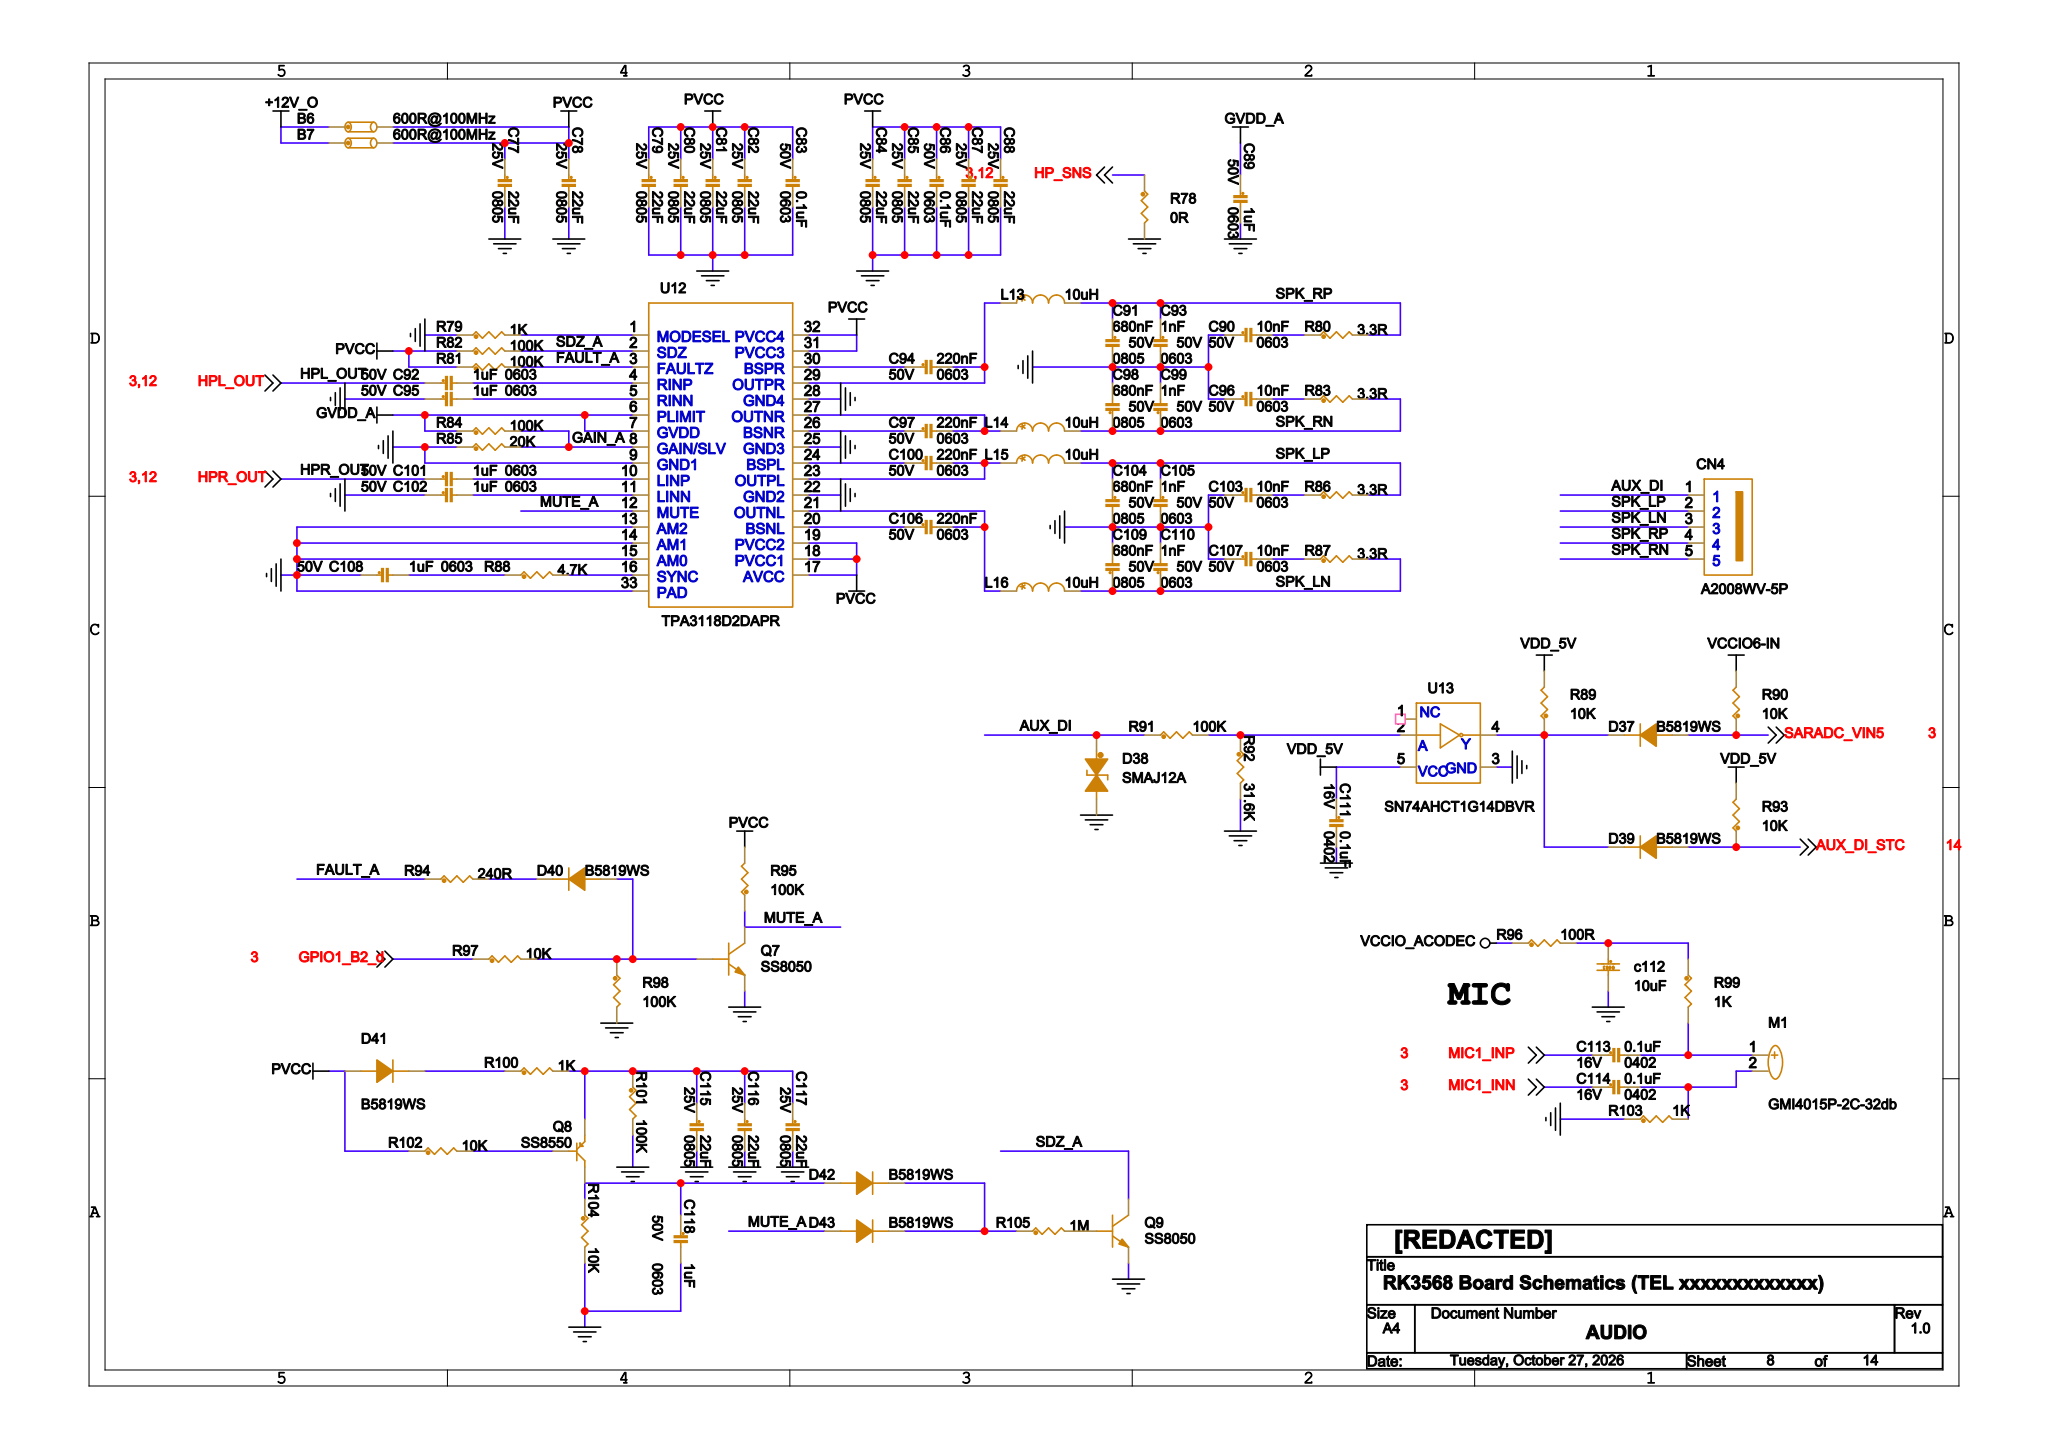Circuit board | Cadence Allegro | 669 parts | 581 nets | one sheet of the schematic
Parts on this sheet (reference | value | footprint):
B6 | 600R@100MHz | R0805
B7 | 600R@100MHz | R0805
C77 | 22uF | C0805
C78 | 22uF | C0805
C79 | 22uF | C0805
C80 | 22uF | C0805
C81 | 22uF | C0805
C82 | 22uF | C0805
C83 | 0.1uF | C0603
C84 | 22uF | C0805
C85 | 22uF | C0805
C86 | 0.1uF | C0603
C87 | 22uF | C0805
C88 | 22uF | C0805
C89 | 1uF | C0603
C90 | 10nF | C0603
C91 | 680nF | C0805
C92 | 1uF | C0603
C93 | 1nF | C0603
C94 | 220nF | C0603
C95 | 1uF | C0603
C96 | 10nF | C0603
C97 | 220nF | C0603
C98 | 680nF | C0805
C99 | 1nF | C0603
C100 | 220nF | C0603
C101 | 1uF | C0603
C102 | 1uF | C0603
C103 | 10nF | C0603
C104 | 680nF | C0805
C105 | 1nF | C0603
C106 | 220nF | C0603
C107 | 10nF | C0603
C108 | 1uF | C0603
C109 | 680nF | C0805
C110 | 1nF | C0603
C111 | 0.1uF | C0402
C113 | 0.1uF | C0402
C114 | 0.1uF | C0402
C115 | 22uF | C0805
C116 | 22uF | C0805
C117 | 22uF | C0805
C118 | 1uF | C0603
CN4 | A2008WV-5P | A2008WV_5P
D37 | B5819WS | SOD323
D38 | SMAJ12A | SMA
D39 | B5819WS | SOD323
D40 | B5819WS | SOD323
D41 | B5819WS | SOD323
D42 | B5819WS | SOD323
D43 | B5819WS | SOD323
L13 | 10uH | IND0630
L14 | 10uH | IND0630
L15 | 10uH | IND0630
L16 | 10uH | IND0630
M1 | GMI4015P-2C-32db | MIC4015P
Q7 | SS8050 | SOT-23
Q8 | SS8550 | SOT-23
Q9 | SS8050 | SOT-23
R78 | 0R | R0402
R79 | 1K | R0402
R80 | 3.3R | R0603
R81 | 100K | R0402
R82 | 100K | R0402
R83 | 3.3R | R0603
R84 | 100K | R0402
R85 | 20K | R0402
R86 | 3.3R | R0603
R87 | 3.3R | R0603
R88 | 4.7K | R0402
R89 | 10K | R0402
R90 | 10K | R0402
R91 | 100K | R0402
R92 | 31.6K | R0402
R93 | 10K | R0402
R94 | 240R | R0402
R95 | 100K | R0402
R96 | 100R | R0402
R97 | 10K | R0402
R98 | 100K | R0402
R99 | 1K | R0402
R100 | 1K | R0402
R101 | 100K | R0402
R102 | 10K | R0402
R103 | 1K | R0402
R104 | 10K | R0402
R105 | 1M | R0402
U12 | TPA3118D2DAPR | HTSSOP32
U13 | SN74AHCT1G14DBVR | SOT23-5
Nets of these parts (net: part-pin ...):
GND: C77-2 C78-2 C79-2 C80-2 C81-2 C82-2 C83-2 C84-2 C85-2 C86-2 C87-2 C88-2 C89-2 C90-1 C91-2 C93-2 C95-1 C96-1 C98-2 C99-2 C102-1 C103-1 C104-2 C105-2 C107-1 C108-1 C109-2 C110-2 C111-2 C115-2 C116-2 C117-2 C118-2 D38-1 Q7-2 Q9-2 R78-2 R79-1 R85-1 R92-2 R98-2 R101-2 R103-1 R104-2 U13-3 U12-9 U12-13 U12-14 U12-15 U12-22 U12-25 U12-28 U12-33
VDD_5V: C111-1 R89-2 R93-2 U13-5
+12V_O: B6-1 B7-1
SARADC_VIN5: D37-1 R90-1
N84592659: D37-2 D39-2 R89-1 U13-4
AUX_DI_STC: D39-1 R93-1
N84585289: D40-1 Q7-1 R97-2 R98-1
N84585271: D40-2 R94-2
PVCC: B6-2 B7-2 C77-1 C78-1 C79-1 C80-1 C81-1 C82-1 C83-1 C84-1 C85-1 C86-1 C87-1 C88-1 D41-1 R81-1 R82-1 R95-2 R102-1 U12-17 U12-18 U12-19 U12-31 U12-32
N84584641: D41-2 R100-1
N84584680: C118-1 D42-1 Q8-3 R104-1
N84584795: D42-2 D43-2 R105-1
MUTE_A: D43-1 Q7-3 R95-1 U12-12
N84323691: C113-2 M1-1 R99-2
N84323732: C114-2 M1-2 R103-2
VCCIO6-IN: R90-2
HPR_OUT: C101-1
N84586479: C101-2 U12-10
N84586481: C102-2 U12-11
N84586513: C108-2 R88-1
HPL_OUT: C92-1
GVDD_A: C89-1 R84-1 U12-6 U12-7
N84586375: C92-2 U12-4
N84586397: C95-2 U12-5
N84586869: C103-2 R86-1
N84586851: C107-2 R87-1
N84586809: C90-2 R80-1
N84586807: C96-2 R83-1
SPK_LP: C104-1 C105-1 CN4-2 L15-2 R86-2
SPK_LN: C109-1 C110-1 CN4-3 L16-2 R87-2
SPK_RP: C91-1 C93-1 CN4-4 L13-2 R80-2
SPK_RN: C98-1 C99-1 CN4-5 L14-2 R83-2
N84586637: C106-1 U12-20
N84586639: C106-2 L16-1 U12-21
N84586605: C94-1 U12-30
N84586607: C94-2 L13-1 U12-29
N84586623: C97-1 U12-26
N84586625: C97-2 L14-1 U12-27
N84586629: C100-1 U12-24
N84586631: C100-2 L15-1 U12-23
MIC1_INP: C113-1
MIC1_INN: C114-1
N84584652: C115-1 C116-1 C117-1 Q8-2 R100-2 R101-1
AUX_DI: CN4-1 D38-2 R91-1
N845848051: Q9-1 R105-2
SDZ_A: Q9-3 R82-2 U12-2
N84584670: Q8-1 R102-2
HP_SNS: R78-1
GPIO1_B2_D: R97-1
GAIN_A: R84-2 R85-2 U12-8
VCCIO_ACODEC: R96-1
N84323697: R96-2 R99-1
FAULT_A: R81-2 R94-1 U12-3
N84592769: R91-2 R92-1 U13-2
N84586325: R79-2 U12-1
N84586515: R88-2 U12-16